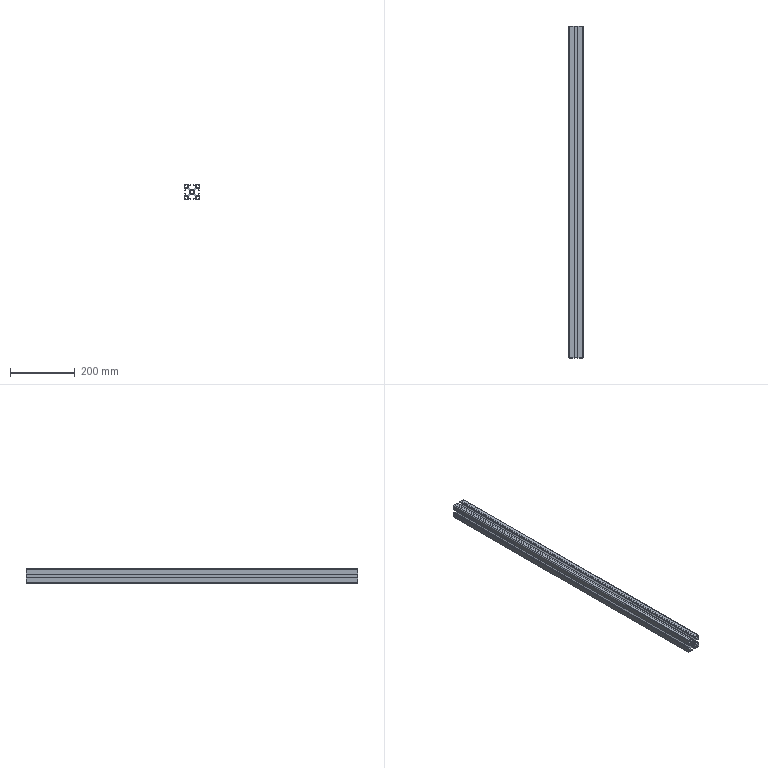Part | STEP file | 1 solid | 135 faces | box 45 x 1022 x 45 mm | volume 707174 mm3 | plane 118 | cylinder 17 | commonest cylinder face diameters 10 x9 3 x4 5 x4